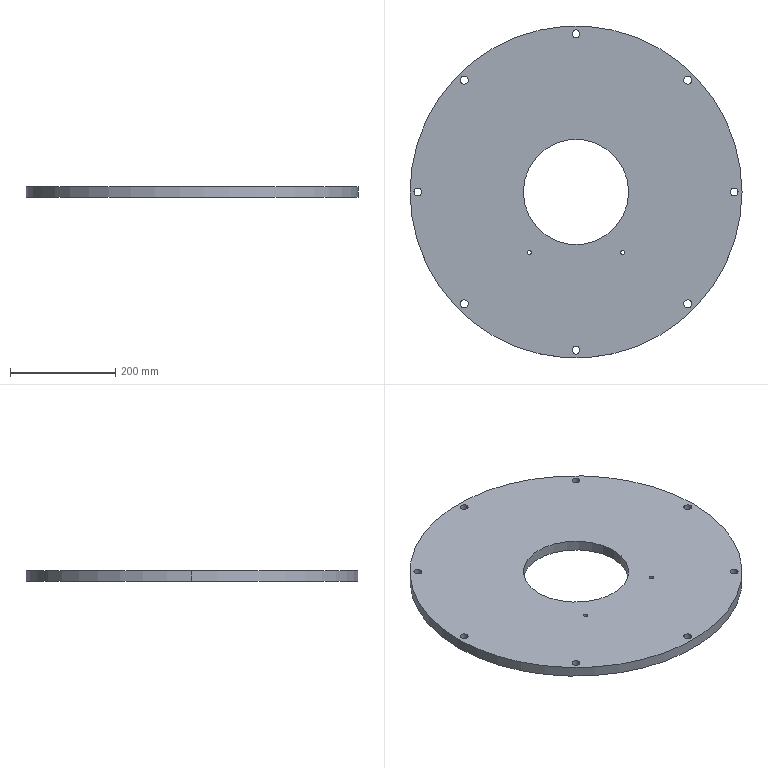Part | SolidWorks | features Cut 1, Extrusion 1 | 1 solid | 26 faces | box 630 x 630 x 20 mm | volume 5575887 mm3 | cylinder 24 | plane 2 | commonest cylinder face diameters 15 x16 8 x4 200 x2 630 x2
STEP:
#1=CARTESIAN_POINT('',(84.459,-114.891,20.));
#2=VERTEX_POINT('',#1);
#3=CARTESIAN_POINT('',(92.459,-114.891,20.));
#4=VERTEX_POINT('',#3);
#5=CARTESIAN_POINT('',(88.459,-114.891,20.));
#6=DIRECTION('',(0.,0.,1.));
#7=DIRECTION('',(1.,0.,0.));
#8=AXIS2_PLACEMENT_3D('',#5,#6,#7);
#9=CIRCLE('',#8,4.);
#10=EDGE_CURVE('',#2,#4,#9,.T.);
#11=ORIENTED_EDGE('',*,*,#10,.T.);
#12=CARTESIAN_POINT('',(92.459,-114.891,0.));
#13=VERTEX_POINT('',#12);
#14=CARTESIAN_POINT('',(92.459,-114.891,50.));
#15=DIRECTION('',(0.,0.,-1.));
#16=VECTOR('',#15,1000.);
#17=LINE('',#14,#16);
#18=EDGE_CURVE('',#4,#13,#17,.T.);
#19=ORIENTED_EDGE('',*,*,#18,.T.);
#20=CARTESIAN_POINT('',(84.459,-114.891,0.));
#21=VERTEX_POINT('',#20);
#22=CARTESIAN_POINT('',(88.459,-114.891,0.));
#23=DIRECTION('',(0.,0.,-1.));
#24=DIRECTION('',(-1.,0.,0.));
#25=AXIS2_PLACEMENT_3D('',#22,#23,#24);
#26=CIRCLE('',#25,4.);
#27=EDGE_CURVE('',#13,#21,#26,.T.);
#28=ORIENTED_EDGE('',*,*,#27,.T.);
#29=CARTESIAN_POINT('',(84.459,-114.891,50.));
#30=DIRECTION('',(0.,0.,-1.));
#31=VECTOR('',#30,1000.);
#32=LINE('',#29,#31);
#33=EDGE_CURVE('',#2,#21,#32,.T.);
#34=ORIENTED_EDGE('',*,*,#33,.F.);
#35=EDGE_LOOP('',(#11,#19,#28,#34));
#36=FACE_OUTER_BOUND('',#35,.T.);
#37=CARTESIAN_POINT('',(88.459,-114.891,50.));
#38=DIRECTION('',(0.,0.,-1.));
#39=DIRECTION('',(-1.,0.,0.));
#40=AXIS2_PLACEMENT_3D('',#37,#38,#39);
#41=CYLINDRICAL_SURFACE('',#40,4.);
#42=ADVANCED_FACE('',(#36),#41,.F.);
#43=CARTESIAN_POINT('',(-92.459,-114.891,20.));
#44=VERTEX_POINT('',#43);
#45=CARTESIAN_POINT('',(-84.459,-114.891,20.));
#46=VERTEX_POINT('',#45);
#47=CARTESIAN_POINT('',(-88.459,-114.891,20.));
#48=DIRECTION('',(0.,0.,1.));
#49=DIRECTION('',(1.,0.,0.));
#50=AXIS2_PLACEMENT_3D('',#47,#48,#49);
#51=CIRCLE('',#50,4.);
#52=EDGE_CURVE('',#44,#46,#51,.T.);
#53=ORIENTED_EDGE('',*,*,#52,.T.);
#54=CARTESIAN_POINT('',(-84.459,-114.891,0.));
#55=VERTEX_POINT('',#54);
#56=CARTESIAN_POINT('',(-84.459,-114.891,50.));
#57=DIRECTION('',(0.,0.,-1.));
#58=VECTOR('',#57,1000.);
#59=LINE('',#56,#58);
#60=EDGE_CURVE('',#46,#55,#59,.T.);
#61=ORIENTED_EDGE('',*,*,#60,.T.);
#62=CARTESIAN_POINT('',(-92.459,-114.891,0.));
#63=VERTEX_POINT('',#62);
#64=CARTESIAN_POINT('',(-88.459,-114.891,0.));
#65=DIRECTION('',(0.,0.,-1.));
#66=DIRECTION('',(-1.,0.,0.));
#67=AXIS2_PLACEMENT_3D('',#64,#65,#66);
#68=CIRCLE('',#67,4.);
#69=EDGE_CURVE('',#55,#63,#68,.T.);
#70=ORIENTED_EDGE('',*,*,#69,.T.);
#71=CARTESIAN_POINT('',(-92.459,-114.891,50.));
#72=DIRECTION('',(0.,0.,-1.));
#73=VECTOR('',#72,1000.);
#74=LINE('',#71,#73);
#75=EDGE_CURVE('',#44,#63,#74,.T.);
#76=ORIENTED_EDGE('',*,*,#75,.F.);
#77=EDGE_LOOP('',(#53,#61,#70,#76));
#78=FACE_OUTER_BOUND('',#77,.T.);
#79=CARTESIAN_POINT('',(-88.459,-114.891,50.));
#80=DIRECTION('',(0.,0.,-1.));
#81=DIRECTION('',(-1.,0.,0.));
#82=AXIS2_PLACEMENT_3D('',#79,#80,#81);
#83=CYLINDRICAL_SURFACE('',#82,4.);
#84=ADVANCED_FACE('',(#78),#83,.F.);
#85=CARTESIAN_POINT('',(-219.632,212.132,20.));
#86=VERTEX_POINT('',#85);
#87=CARTESIAN_POINT('',(-204.632,212.132,20.));
#88=VERTEX_POINT('',#87);
#89=CARTESIAN_POINT('',(-212.132,212.132,20.));
#90=DIRECTION('',(0.,0.,1.));
#91=DIRECTION('',(1.,0.,0.));
#92=AXIS2_PLACEMENT_3D('',#89,#90,#91);
#93=CIRCLE('',#92,7.5);
#94=EDGE_CURVE('',#86,#88,#93,.T.);
#95=ORIENTED_EDGE('',*,*,#94,.T.);
#96=CARTESIAN_POINT('',(-204.632,212.132,0.));
#97=VERTEX_POINT('',#96);
#98=CARTESIAN_POINT('',(-204.632,212.132,20.));
#99=DIRECTION('',(0.,0.,-1.));
#100=VECTOR('',#99,1000.);
#101=LINE('',#98,#100);
#102=EDGE_CURVE('',#88,#97,#101,.T.);
#103=ORIENTED_EDGE('',*,*,#102,.T.);
#104=CARTESIAN_POINT('',(-219.632,212.132,0.));
#105=VERTEX_POINT('',#104);
#106=CARTESIAN_POINT('',(-212.132,212.132,0.));
#107=DIRECTION('',(0.,0.,1.));
#108=DIRECTION('',(1.,0.,0.));
#109=AXIS2_PLACEMENT_3D('',#106,#107,#108);
#110=CIRCLE('',#109,7.5);
#111=EDGE_CURVE('',#105,#97,#110,.T.);
#112=ORIENTED_EDGE('',*,*,#111,.F.);
#113=CARTESIAN_POINT('',(-219.632,212.132,20.));
#114=DIRECTION('',(0.,0.,-1.));
#115=VECTOR('',#114,1000.);
#116=LINE('',#113,#115);
#117=EDGE_CURVE('',#86,#105,#116,.T.);
#118=ORIENTED_EDGE('',*,*,#117,.F.);
#119=EDGE_LOOP('',(#95,#103,#112,#118));
#120=FACE_OUTER_BOUND('',#119,.T.);
#121=CARTESIAN_POINT('',(-212.132,212.132,20.));
#122=DIRECTION('',(0.,0.,-1.));
#123=DIRECTION('',(-1.,0.,0.));
#124=AXIS2_PLACEMENT_3D('',#121,#122,#123);
#125=CYLINDRICAL_SURFACE('',#124,7.5);
#126=ADVANCED_FACE('',(#120),#125,.F.);
#127=CARTESIAN_POINT('',(-307.5,0.,20.));
#128=VERTEX_POINT('',#127);
#129=CARTESIAN_POINT('',(-292.5,0.,20.));
#130=VERTEX_POINT('',#129);
#131=CARTESIAN_POINT('',(-300.,0.,20.));
#132=DIRECTION('',(0.,0.,1.));
#133=DIRECTION('',(1.,0.,0.));
#134=AXIS2_PLACEMENT_3D('',#131,#132,#133);
#135=CIRCLE('',#134,7.5);
#136=EDGE_CURVE('',#128,#130,#135,.T.);
#137=ORIENTED_EDGE('',*,*,#136,.T.);
#138=CARTESIAN_POINT('',(-292.5,0.,0.));
#139=VERTEX_POINT('',#138);
#140=CARTESIAN_POINT('',(-292.5,0.,20.));
#141=DIRECTION('',(0.,0.,-1.));
#142=VECTOR('',#141,1000.);
#143=LINE('',#140,#142);
#144=EDGE_CURVE('',#130,#139,#143,.T.);
#145=ORIENTED_EDGE('',*,*,#144,.T.);
#146=CARTESIAN_POINT('',(-307.5,0.,0.));
#147=VERTEX_POINT('',#146);
#148=CARTESIAN_POINT('',(-300.,0.,0.));
#149=DIRECTION('',(0.,0.,1.));
#150=DIRECTION('',(1.,0.,0.));
#151=AXIS2_PLACEMENT_3D('',#148,#149,#150);
#152=CIRCLE('',#151,7.5);
#153=EDGE_CURVE('',#147,#139,#152,.T.);
#154=ORIENTED_EDGE('',*,*,#153,.F.);
#155=CARTESIAN_POINT('',(-307.5,0.,20.));
#156=DIRECTION('',(0.,0.,-1.));
#157=VECTOR('',#156,1000.);
#158=LINE('',#155,#157);
#159=EDGE_CURVE('',#128,#147,#158,.T.);
#160=ORIENTED_EDGE('',*,*,#159,.F.);
#161=EDGE_LOOP('',(#137,#145,#154,#160));
#162=FACE_OUTER_BOUND('',#161,.T.);
#163=CARTESIAN_POINT('',(-300.,0.,20.));
#164=DIRECTION('',(0.,0.,-1.));
#165=DIRECTION('',(-1.,0.,0.));
#166=AXIS2_PLACEMENT_3D('',#163,#164,#165);
#167=CYLINDRICAL_SURFACE('',#166,7.5);
#168=ADVANCED_FACE('',(#162),#167,.F.);
#169=CARTESIAN_POINT('',(-219.632,-212.132,20.));
#170=VERTEX_POINT('',#169);
#171=CARTESIAN_POINT('',(-204.632,-212.132,20.));
#172=VERTEX_POINT('',#171);
#173=CARTESIAN_POINT('',(-212.132,-212.132,20.));
#174=DIRECTION('',(0.,0.,1.));
#175=DIRECTION('',(1.,0.,0.));
#176=AXIS2_PLACEMENT_3D('',#173,#174,#175);
#177=CIRCLE('',#176,7.5);
#178=EDGE_CURVE('',#170,#172,#177,.T.);
#179=ORIENTED_EDGE('',*,*,#178,.T.);
#180=CARTESIAN_POINT('',(-204.632,-212.132,0.));
#181=VERTEX_POINT('',#180);
#182=CARTESIAN_POINT('',(-204.632,-212.132,20.));
#183=DIRECTION('',(0.,0.,-1.));
#184=VECTOR('',#183,1000.);
#185=LINE('',#182,#184);
#186=EDGE_CURVE('',#172,#181,#185,.T.);
#187=ORIENTED_EDGE('',*,*,#186,.T.);
#188=CARTESIAN_POINT('',(-219.632,-212.132,0.));
#189=VERTEX_POINT('',#188);
#190=CARTESIAN_POINT('',(-212.132,-212.132,0.));
#191=DIRECTION('',(0.,0.,1.));
#192=DIRECTION('',(1.,0.,0.));
#193=AXIS2_PLACEMENT_3D('',#190,#191,#192);
#194=CIRCLE('',#193,7.5);
#195=EDGE_CURVE('',#189,#181,#194,.T.);
#196=ORIENTED_EDGE('',*,*,#195,.F.);
#197=CARTESIAN_POINT('',(-219.632,-212.132,20.));
#198=DIRECTION('',(0.,0.,-1.));
#199=VECTOR('',#198,1000.);
#200=LINE('',#197,#199);
#201=EDGE_CURVE('',#170,#189,#200,.T.);
#202=ORIENTED_EDGE('',*,*,#201,.F.);
#203=EDGE_LOOP('',(#179,#187,#196,#202));
#204=FACE_OUTER_BOUND('',#203,.T.);
#205=CARTESIAN_POINT('',(-212.132,-212.132,20.));
#206=DIRECTION('',(0.,0.,-1.));
#207=DIRECTION('',(-1.,0.,0.));
#208=AXIS2_PLACEMENT_3D('',#205,#206,#207);
#209=CYLINDRICAL_SURFACE('',#208,7.5);
#210=ADVANCED_FACE('',(#204),#209,.F.);
#211=CARTESIAN_POINT('',(-7.5,-300.,20.));
#212=VERTEX_POINT('',#211);
#213=CARTESIAN_POINT('',(7.5,-300.,20.));
#214=VERTEX_POINT('',#213);
#215=CARTESIAN_POINT('',(0.,-300.,20.));
#216=DIRECTION('',(0.,0.,1.));
#217=DIRECTION('',(1.,0.,0.));
#218=AXIS2_PLACEMENT_3D('',#215,#216,#217);
#219=CIRCLE('',#218,7.5);
#220=EDGE_CURVE('',#212,#214,#219,.T.);
#221=ORIENTED_EDGE('',*,*,#220,.T.);
#222=CARTESIAN_POINT('',(7.5,-300.,0.));
#223=VERTEX_POINT('',#222);
#224=CARTESIAN_POINT('',(7.5,-300.,20.));
#225=DIRECTION('',(0.,0.,-1.));
#226=VECTOR('',#225,1000.);
#227=LINE('',#224,#226);
#228=EDGE_CURVE('',#214,#223,#227,.T.);
#229=ORIENTED_EDGE('',*,*,#228,.T.);
#230=CARTESIAN_POINT('',(-7.5,-300.,0.));
#231=VERTEX_POINT('',#230);
#232=CARTESIAN_POINT('',(0.,-300.,0.));
#233=DIRECTION('',(0.,0.,1.));
#234=DIRECTION('',(1.,0.,0.));
#235=AXIS2_PLACEMENT_3D('',#232,#233,#234);
#236=CIRCLE('',#235,7.5);
#237=EDGE_CURVE('',#231,#223,#236,.T.);
#238=ORIENTED_EDGE('',*,*,#237,.F.);
#239=CARTESIAN_POINT('',(-7.5,-300.,20.));
#240=DIRECTION('',(0.,0.,-1.));
#241=VECTOR('',#240,1000.);
#242=LINE('',#239,#241);
#243=EDGE_CURVE('',#212,#231,#242,.T.);
#244=ORIENTED_EDGE('',*,*,#243,.F.);
#245=EDGE_LOOP('',(#221,#229,#238,#244));
#246=FACE_OUTER_BOUND('',#245,.T.);
#247=CARTESIAN_POINT('',(0.,-300.,20.));
#248=DIRECTION('',(0.,0.,-1.));
#249=DIRECTION('',(-1.,0.,0.));
#250=AXIS2_PLACEMENT_3D('',#247,#248,#249);
#251=CYLINDRICAL_SURFACE('',#250,7.5);
#252=ADVANCED_FACE('',(#246),#251,.F.);
#253=CARTESIAN_POINT('',(204.632,-212.132,20.));
#254=VERTEX_POINT('',#253);
#255=CARTESIAN_POINT('',(219.632,-212.132,20.));
#256=VERTEX_POINT('',#255);
#257=CARTESIAN_POINT('',(212.132,-212.132,20.));
#258=DIRECTION('',(0.,0.,1.));
#259=DIRECTION('',(1.,0.,0.));
#260=AXIS2_PLACEMENT_3D('',#257,#258,#259);
#261=CIRCLE('',#260,7.5);
#262=EDGE_CURVE('',#254,#256,#261,.T.);
#263=ORIENTED_EDGE('',*,*,#262,.T.);
#264=CARTESIAN_POINT('',(219.632,-212.132,0.));
#265=VERTEX_POINT('',#264);
#266=CARTESIAN_POINT('',(219.632,-212.132,20.));
#267=DIRECTION('',(0.,0.,-1.));
#268=VECTOR('',#267,1000.);
#269=LINE('',#266,#268);
#270=EDGE_CURVE('',#256,#265,#269,.T.);
#271=ORIENTED_EDGE('',*,*,#270,.T.);
#272=CARTESIAN_POINT('',(204.632,-212.132,0.));
#273=VERTEX_POINT('',#272);
#274=CARTESIAN_POINT('',(212.132,-212.132,0.));
#275=DIRECTION('',(0.,0.,1.));
#276=DIRECTION('',(1.,0.,0.));
#277=AXIS2_PLACEMENT_3D('',#274,#275,#276);
#278=CIRCLE('',#277,7.5);
#279=EDGE_CURVE('',#273,#265,#278,.T.);
#280=ORIENTED_EDGE('',*,*,#279,.F.);
#281=CARTESIAN_POINT('',(204.632,-212.132,20.));
#282=DIRECTION('',(0.,0.,-1.));
#283=VECTOR('',#282,1000.);
#284=LINE('',#281,#283);
#285=EDGE_CURVE('',#254,#273,#284,.T.);
#286=ORIENTED_EDGE('',*,*,#285,.F.);
#287=EDGE_LOOP('',(#263,#271,#280,#286));
#288=FACE_OUTER_BOUND('',#287,.T.);
#289=CARTESIAN_POINT('',(212.132,-212.132,20.));
#290=DIRECTION('',(0.,0.,-1.));
#291=DIRECTION('',(-1.,0.,0.));
#292=AXIS2_PLACEMENT_3D('',#289,#290,#291);
#293=CYLINDRICAL_SURFACE('',#292,7.5);
#294=ADVANCED_FACE('',(#288),#293,.F.);
#295=CARTESIAN_POINT('',(292.5,0.,20.));
#296=VERTEX_POINT('',#295);
#297=CARTESIAN_POINT('',(307.5,0.,20.));
#298=VERTEX_POINT('',#297);
#299=CARTESIAN_POINT('',(300.,0.,20.));
#300=DIRECTION('',(0.,0.,1.));
#301=DIRECTION('',(1.,0.,0.));
#302=AXIS2_PLACEMENT_3D('',#299,#300,#301);
#303=CIRCLE('',#302,7.5);
#304=EDGE_CURVE('',#296,#298,#303,.T.);
#305=ORIENTED_EDGE('',*,*,#304,.T.);
#306=CARTESIAN_POINT('',(307.5,0.,0.));
#307=VERTEX_POINT('',#306);
#308=CARTESIAN_POINT('',(307.5,0.,20.));
#309=DIRECTION('',(0.,0.,-1.));
#310=VECTOR('',#309,1000.);
#311=LINE('',#308,#310);
#312=EDGE_CURVE('',#298,#307,#311,.T.);
#313=ORIENTED_EDGE('',*,*,#312,.T.);
#314=CARTESIAN_POINT('',(292.5,0.,0.));
#315=VERTEX_POINT('',#314);
#316=CARTESIAN_POINT('',(300.,0.,0.));
#317=DIRECTION('',(0.,0.,1.));
#318=DIRECTION('',(1.,0.,0.));
#319=AXIS2_PLACEMENT_3D('',#316,#317,#318);
#320=CIRCLE('',#319,7.5);
#321=EDGE_CURVE('',#315,#307,#320,.T.);
#322=ORIENTED_EDGE('',*,*,#321,.F.);
#323=CARTESIAN_POINT('',(292.5,0.,20.));
#324=DIRECTION('',(0.,0.,-1.));
#325=VECTOR('',#324,1000.);
#326=LINE('',#323,#325);
#327=EDGE_CURVE('',#296,#315,#326,.T.);
#328=ORIENTED_EDGE('',*,*,#327,.F.);
#329=EDGE_LOOP('',(#305,#313,#322,#328));
#330=FACE_OUTER_BOUND('',#329,.T.);
#331=CARTESIAN_POINT('',(300.,0.,20.));
#332=DIRECTION('',(0.,0.,-1.));
#333=DIRECTION('',(-1.,0.,0.));
#334=AXIS2_PLACEMENT_3D('',#331,#332,#333);
#335=CYLINDRICAL_SURFACE('',#334,7.5);
#336=ADVANCED_FACE('',(#330),#335,.F.);
#337=CARTESIAN_POINT('',(204.632,212.132,20.));
#338=VERTEX_POINT('',#337);
#339=CARTESIAN_POINT('',(219.632,212.132,20.));
#340=VERTEX_POINT('',#339);
#341=CARTESIAN_POINT('',(212.132,212.132,20.));
#342=DIRECTION('',(0.,0.,1.));
#343=DIRECTION('',(1.,0.,0.));
#344=AXIS2_PLACEMENT_3D('',#341,#342,#343);
#345=CIRCLE('',#344,7.5);
#346=EDGE_CURVE('',#338,#340,#345,.T.);
#347=ORIENTED_EDGE('',*,*,#346,.T.);
#348=CARTESIAN_POINT('',(219.632,212.132,0.));
#349=VERTEX_POINT('',#348);
#350=CARTESIAN_POINT('',(219.632,212.132,20.));
#351=DIRECTION('',(0.,0.,-1.));
#352=VECTOR('',#351,1000.);
#353=LINE('',#350,#352);
#354=EDGE_CURVE('',#340,#349,#353,.T.);
#355=ORIENTED_EDGE('',*,*,#354,.T.);
#356=CARTESIAN_POINT('',(204.632,212.132,0.));
#357=VERTEX_POINT('',#356);
#358=CARTESIAN_POINT('',(212.132,212.132,0.));
#359=DIRECTION('',(0.,0.,1.));
#360=DIRECTION('',(1.,0.,0.));
#361=AXIS2_PLACEMENT_3D('',#358,#359,#360);
#362=CIRCLE('',#361,7.5);
#363=EDGE_CURVE('',#357,#349,#362,.T.);
#364=ORIENTED_EDGE('',*,*,#363,.F.);
#365=CARTESIAN_POINT('',(204.632,212.132,20.));
#366=DIRECTION('',(0.,0.,-1.));
#367=VECTOR('',#366,1000.);
#368=LINE('',#365,#367);
#369=EDGE_CURVE('',#338,#357,#368,.T.);
#370=ORIENTED_EDGE('',*,*,#369,.F.);
#371=EDGE_LOOP('',(#347,#355,#364,#370));
#372=FACE_OUTER_BOUND('',#371,.T.);
#373=CARTESIAN_POINT('',(212.132,212.132,20.));
#374=DIRECTION('',(0.,0.,-1.));
#375=DIRECTION('',(-1.,0.,0.));
#376=AXIS2_PLACEMENT_3D('',#373,#374,#375);
#377=CYLINDRICAL_SURFACE('',#376,7.5);
#378=ADVANCED_FACE('',(#372),#377,.F.);
#379=CARTESIAN_POINT('',(-7.5,300.,20.));
#380=VERTEX_POINT('',#379);
#381=CARTESIAN_POINT('',(7.5,300.,20.));
#382=VERTEX_POINT('',#381);
#383=CARTESIAN_POINT('',(0.,300.,20.));
#384=DIRECTION('',(0.,0.,1.));
#385=DIRECTION('',(1.,0.,0.));
#386=AXIS2_PLACEMENT_3D('',#383,#384,#385);
#387=CIRCLE('',#386,7.5);
#388=EDGE_CURVE('',#380,#382,#387,.T.);
#389=ORIENTED_EDGE('',*,*,#388,.T.);
#390=CARTESIAN_POINT('',(7.5,300.,0.));
#391=VERTEX_POINT('',#390);
#392=CARTESIAN_POINT('',(7.5,300.,20.));
#393=DIRECTION('',(0.,0.,-1.));
#394=VECTOR('',#393,1000.);
#395=LINE('',#392,#394);
#396=EDGE_CURVE('',#382,#391,#395,.T.);
#397=ORIENTED_EDGE('',*,*,#396,.T.);
#398=CARTESIAN_POINT('',(-7.5,300.,0.));
#399=VERTEX_POINT('',#398);
#400=CARTESIAN_POINT('',(0.,300.,0.));
#401=DIRECTION('',(0.,0.,1.));
#402=DIRECTION('',(1.,0.,0.));
#403=AXIS2_PLACEMENT_3D('',#400,#401,#402);
#404=CIRCLE('',#403,7.5);
#405=EDGE_CURVE('',#399,#391,#404,.T.);
#406=ORIENTED_EDGE('',*,*,#405,.F.);
#407=CARTESIAN_POINT('',(-7.5,300.,20.));
#408=DIRECTION('',(0.,0.,-1.));
#409=VECTOR('',#408,1000.);
#410=LINE('',#407,#409);
#411=EDGE_CURVE('',#380,#399,#410,.T.);
#412=ORIENTED_EDGE('',*,*,#411,.F.);
#413=EDGE_LOOP('',(#389,#397,#406,#412));
#414=FACE_OUTER_BOUND('',#413,.T.);
#415=CARTESIAN_POINT('',(0.,300.,20.));
#416=DIRECTION('',(0.,0.,-1.));
#417=DIRECTION('',(-1.,0.,0.));
#418=AXIS2_PLACEMENT_3D('',#415,#416,#417);
#419=CYLINDRICAL_SURFACE('',#418,7.5);
#420=ADVANCED_FACE('',(#414),#419,.F.);
#421=CARTESIAN_POINT('',(-100.,0.,20.));
#422=VERTEX_POINT('',#421);
#423=CARTESIAN_POINT('',(100.,0.,20.));
#424=VERTEX_POINT('',#423);
#425=CARTESIAN_POINT('',(0.,0.,20.));
#426=DIRECTION('',(0.,0.,1.));
#427=DIRECTION('',(1.,0.,0.));
#428=AXIS2_PLACEMENT_3D('',#425,#426,#427);
#429=CIRCLE('',#428,100.);
#430=EDGE_CURVE('',#422,#424,#429,.T.);
#431=ORIENTED_EDGE('',*,*,#430,.T.);
#432=CARTESIAN_POINT('',(100.,0.,0.));
#433=VERTEX_POINT('',#432);
#434=CARTESIAN_POINT('',(100.,0.,20.));
#435=DIRECTION('',(0.,0.,-1.));
#436=VECTOR('',#435,1000.);
#437=LINE('',#434,#436);
#438=EDGE_CURVE('',#424,#433,#437,.T.);
#439=ORIENTED_EDGE('',*,*,#438,.T.);
#440=CARTESIAN_POINT('',(-100.,0.,0.));
#441=VERTEX_POINT('',#440);
#442=CARTESIAN_POINT('',(0.,0.,0.));
#443=DIRECTION('',(0.,0.,1.));
#444=DIRECTION('',(1.,0.,0.));
#445=AXIS2_PLACEMENT_3D('',#442,#443,#444);
#446=CIRCLE('',#445,100.);
#447=EDGE_CURVE('',#441,#433,#446,.T.);
#448=ORIENTED_EDGE('',*,*,#447,.F.);
#449=CARTESIAN_POINT('',(-100.,0.,20.));
#450=DIRECTION('',(0.,0.,-1.));
#451=VECTOR('',#450,1000.);
#452=LINE('',#449,#451);
#453=EDGE_CURVE('',#422,#441,#452,.T.);
#454=ORIENTED_EDGE('',*,*,#453,.F.);
#455=EDGE_LOOP('',(#431,#439,#448,#454));
#456=FACE_OUTER_BOUND('',#455,.T.);
#457=CARTESIAN_POINT('',(0.,0.,20.));
#458=DIRECTION('',(0.,0.,-1.));
#459=DIRECTION('',(-1.,0.,0.));
#460=AXIS2_PLACEMENT_3D('',#457,#458,#459);
#461=CYLINDRICAL_SURFACE('',#460,100.);
#462=ADVANCED_FACE('',(#456),#461,.F.);
#463=CARTESIAN_POINT('',(315.,0.,20.));
#464=VERTEX_POINT('',#463);
#465=CARTESIAN_POINT('',(-315.,0.,20.));
#466=VERTEX_POINT('',#465);
#467=CARTESIAN_POINT('',(0.,0.,20.));
#468=DIRECTION('',(0.,0.,1.));
#469=DIRECTION('',(1.,0.,0.));
#470=AXIS2_PLACEMENT_3D('',#467,#468,#469);
#471=CIRCLE('',#470,315.);
#472=EDGE_CURVE('',#464,#466,#471,.T.);
#473=ORIENTED_EDGE('',*,*,#472,.F.);
#474=CARTESIAN_POINT('',(315.,0.,0.));
#475=VERTEX_POINT('',#474);
#476=CARTESIAN_POINT('',(315.,0.,20.));
#477=DIRECTION('',(0.,0.,-1.));
#478=VECTOR('',#477,1000.);
#479=LINE('',#476,#478);
#480=EDGE_CURVE('',#464,#475,#479,.T.);
#481=ORIENTED_EDGE('',*,*,#480,.T.);
#482=CARTESIAN_POINT('',(-315.,0.,0.));
#483=VERTEX_POINT('',#482);
#484=CARTESIAN_POINT('',(0.,0.,0.));
#485=DIRECTION('',(0.,0.,1.));
#486=DIRECTION('',(1.,0.,0.));
#487=AXIS2_PLACEMENT_3D('',#484,#485,#486);
#488=CIRCLE('',#487,315.);
#489=EDGE_CURVE('',#475,#483,#488,.T.);
#490=ORIENTED_EDGE('',*,*,#489,.T.);
#491=CARTESIAN_POINT('',(-315.,0.,20.));
#492=DIRECTION('',(0.,0.,-1.));
#493=VECTOR('',#492,1000.);
#494=LINE('',#491,#493);
#495=EDGE_CURVE('',#466,#483,#494,.T.);
#496=ORIENTED_EDGE('',*,*,#495,.F.);
#497=EDGE_LOOP('',(#473,#481,#490,#496));
#498=FACE_OUTER_BOUND('',#497,.T.);
#499=CARTESIAN_POINT('',(0.,0.,20.));
#500=DIRECTION('',(0.,0.,-1.));
#501=DIRECTION('',(-1.,0.,0.));
#502=AXIS2_PLACEMENT_3D('',#499,#500,#501);
#503=CYLINDRICAL_SURFACE('',#502,315.);
#504=ADVANCED_FACE('',(#498),#503,.T.);
#505=ORIENTED_EDGE('',*,*,#10,.F.);
#506=CARTESIAN_POINT('',(88.459,-114.891,20.));
#507=DIRECTION('',(0.,0.,1.));
#508=DIRECTION('',(1.,0.,0.));
#509=AXIS2_PLACEMENT_3D('',#506,#507,#508);
#510=CIRCLE('',#509,4.);
#511=EDGE_CURVE('',#4,#2,#510,.T.);
#512=ORIENTED_EDGE('',*,*,#511,.F.);
#513=EDGE_LOOP('',(#505,#512));
#514=FACE_BOUND('',#513,.T.);
#515=ORIENTED_EDGE('',*,*,#52,.F.);
#516=CARTESIAN_POINT('',(-88.459,-114.891,20.));
#517=DIRECTION('',(0.,0.,1.));
#518=DIRECTION('',(1.,0.,0.));
#519=AXIS2_PLACEMENT_3D('',#516,#517,#518);
#520=CIRCLE('',#519,4.);
#521=EDGE_CURVE('',#46,#44,#520,.T.);
#522=ORIENTED_EDGE('',*,*,#521,.F.);
#523=EDGE_LOOP('',(#515,#522));
#524=FACE_BOUND('',#523,.T.);
#525=ORIENTED_EDGE('',*,*,#136,.F.);
#526=CARTESIAN_POINT('',(-300.,0.,20.));
#527=DIRECTION('',(0.,0.,1.));
#528=DIRECTION('',(1.,0.,0.));
#529=AXIS2_PLACEMENT_3D('',#526,#527,#528);
#530=CIRCLE('',#529,7.5);
#531=EDGE_CURVE('',#130,#128,#530,.T.);
#532=ORIENTED_EDGE('',*,*,#531,.F.);
#533=EDGE_LOOP('',(#525,#532));
#534=FACE_BOUND('',#533,.T.);
#535=ORIENTED_EDGE('',*,*,#220,.F.);
#536=CARTESIAN_POINT('',(0.,-300.,20.));
#537=DIRECTION('',(0.,0.,1.));
#538=DIRECTION('',(1.,0.,0.));
#539=AXIS2_PLACEMENT_3D('',#536,#537,#538);
#540=CIRCLE('',#539,7.5);
#541=EDGE_CURVE('',#214,#212,#540,.T.);
#542=ORIENTED_EDGE('',*,*,#541,.F.);
#543=EDGE_LOOP('',(#535,#542));
#544=FACE_BOUND('',#543,.T.);
#545=ORIENTED_EDGE('',*,*,#304,.F.);
#546=CARTESIAN_POINT('',(300.,0.,20.));
#547=DIRECTION('',(0.,0.,1.));
#548=DIRECTION('',(1.,0.,0.));
#549=AXIS2_PLACEMENT_3D('',#546,#547,#548);
#550=CIRCLE('',#549,7.5);
#551=EDGE_CURVE('',#298,#296,#550,.T.);
#552=ORIENTED_EDGE('',*,*,#551,.F.);
#553=EDGE_LOOP('',(#545,#552));
#554=FACE_BOUND('',#553,.T.);
#555=ORIENTED_EDGE('',*,*,#388,.F.);
#556=CARTESIAN_POINT('',(0.,300.,20.));
#557=DIRECTION('',(0.,0.,1.));
#558=DIRECTION('',(1.,0.,0.));
#559=AXIS2_PLACEMENT_3D('',#556,#557,#558);
#560=CIRCLE('',#559,7.5);
#561=EDGE_CURVE('',#382,#380,#560,.T.);
#562=ORIENTED_EDGE('',*,*,#561,.F.);
#563=EDGE_LOOP('',(#555,#562));
#564=FACE_BOUND('',#563,.T.);
#565=CARTESIAN_POINT('',(0.,0.,20.));
#566=DIRECTION('',(0.,0.,1.));
#567=DIRECTION('',(1.,0.,0.));
#568=AXIS2_PLACEMENT_3D('',#565,#566,#567);
#569=CIRCLE('',#568,315.);
#570=EDGE_CURVE('',#466,#464,#569,.T.);
#571=ORIENTED_EDGE('',*,*,#570,.T.);
#572=ORIENTED_EDGE('',*,*,#472,.T.);
#573=EDGE_LOOP('',(#571,#572));
#574=FACE_OUTER_BOUND('',#573,.T.);
#575=ORIENTED_EDGE('',*,*,#430,.F.);
#576=CARTESIAN_POINT('',(0.,0.,20.));
#577=DIRECTION('',(0.,0.,1.));
#578=DIRECTION('',(1.,0.,0.));
#579=AXIS2_PLACEMENT_3D('',#576,#577,#578);
#580=CIRCLE('',#579,100.);
#581=EDGE_CURVE('',#424,#422,#580,.T.);
#582=ORIENTED_EDGE('',*,*,#581,.F.);
#583=EDGE_LOOP('',(#575,#582));
#584=FACE_BOUND('',#583,.T.);
#585=ORIENTED_EDGE('',*,*,#346,.F.);
#586=CARTESIAN_POINT('',(212.132,212.132,20.));
#587=DIRECTION('',(0.,0.,1.));
#588=DIRECTION('',(1.,0.,0.));
#589=AXIS2_PLACEMENT_3D('',#586,#587,#588);
#590=CIRCLE('',#589,7.5);
#591=EDGE_CURVE('',#340,#338,#590,.T.);
#592=ORIENTED_EDGE('',*,*,#591,.F.);
#593=EDGE_LOOP('',(#585,#592));
#594=FACE_BOUND('',#593,.T.);
#595=ORIENTED_EDGE('',*,*,#262,.F.);
#596=CARTESIAN_POINT('',(212.132,-212.132,20.));
#597=DIRECTION('',(0.,0.,1.));
#598=DIRECTION('',(1.,0.,0.));
#599=AXIS2_PLACEMENT_3D('',#596,#597,#598);
#600=CIRCLE('',#599,7.5);
#601=EDGE_CURVE('',#256,#254,#600,.T.);
#602=ORIENTED_EDGE('',*,*,#601,.F.);
#603=EDGE_LOOP('',(#595,#602));
#604=FACE_BOUND('',#603,.T.);
#605=ORIENTED_EDGE('',*,*,#178,.F.);
#606=CARTESIAN_POINT('',(-212.132,-212.132,20.));
#607=DIRECTION('',(0.,0.,1.));
#608=DIRECTION('',(1.,0.,0.));
#609=AXIS2_PLACEMENT_3D('',#606,#607,#608);
#610=CIRCLE('',#609,7.5);
#611=EDGE_CURVE('',#172,#170,#610,.T.);
#612=ORIENTED_EDGE('',*,*,#611,.F.);
#613=EDGE_LOOP('',(#605,#612));
#614=FACE_BOUND('',#613,.T.);
#615=ORIENTED_EDGE('',*,*,#94,.F.);
#616=CARTESIAN_POINT('',(-212.132,212.132,20.));
#617=DIRECTION('',(0.,0.,1.));
#618=DIRECTION('',(1.,0.,0.));
#619=AXIS2_PLACEMENT_3D('',#616,#617,#618);
#620=CIRCLE('',#619,7.5);
#621=EDGE_CURVE('',#88,#86,#620,.T.);
#622=ORIENTED_EDGE('',*,*,#621,.F.);
#623=EDGE_LOOP('',(#615,#622));
#624=FACE_BOUND('',#623,.T.);
#625=CARTESIAN_POINT('',(0.,0.,20.));
#626=DIRECTION('',(0.,0.,1.));
#627=DIRECTION('',(1.,0.,0.));
#628=AXIS2_PLACEMENT_3D('',#625,#626,#627);
#629=PLANE('',#628);
#630=ADVANCED_FACE('',(#514,#524,#534,#544,#554,#564,#574,#584,#594,#604,#614,#624),#629,.T.);
#631=CARTESIAN_POINT('',(88.459,-114.891,0.));
#632=DIRECTION('',(0.,0.,-1.));
#633=DIRECTION('',(-1.,0.,0.));
#634=AXIS2_PLACEMENT_3D('',#631,#632,#633);
#635=CIRCLE('',#634,4.);
#636=EDGE_CURVE('',#21,#13,#635,.T.);
#637=ORIENTED_EDGE('',*,*,#636,.F.);
#638=ORIENTED_EDGE('',*,*,#27,.F.);
#639=EDGE_LOOP('',(#637,#638));
#640=FACE_BOUND('',#639,.T.);
#641=CARTESIAN_POINT('',(-88.459,-114.891,0.));
#642=DIRECTION('',(0.,0.,-1.));
#643=DIRECTION('',(-1.,0.,0.));
#644=AXIS2_PLACEMENT_3D('',#641,#642,#643);
#645=CIRCLE('',#644,4.);
#646=EDGE_CURVE('',#63,#55,#645,.T.);
#647=ORIENTED_EDGE('',*,*,#646,.F.);
#648=ORIENTED_EDGE('',*,*,#69,.F.);
#649=EDGE_LOOP('',(#647,#648));
#650=FACE_BOUND('',#649,.T.);
#651=CARTESIAN_POINT('',(0.,0.,0.));
#652=DIRECTION('',(0.,0.,1.));
#653=DIRECTION('',(1.,0.,0.));
#654=AXIS2_PLACEMENT_3D('',#651,#652,#653);
#655=CIRCLE('',#654,315.);
#656=EDGE_CURVE('',#483,#475,#655,.T.);
#657=ORIENTED_EDGE('',*,*,#656,.F.);
#658=ORIENTED_EDGE('',*,*,#489,.F.);
#659=EDGE_LOOP('',(#657,#658));
#660=FACE_OUTER_BOUND('',#659,.T.);
#661=ORIENTED_EDGE('',*,*,#447,.T.);
#662=CARTESIAN_POINT('',(0.,0.,0.));
#663=DIRECTION('',(0.,0.,1.));
#664=DIRECTION('',(1.,0.,0.));
#665=AXIS2_PLACEMENT_3D('',#662,#663,#664);
#666=CIRCLE('',#665,100.);
#667=EDGE_CURVE('',#433,#441,#666,.T.);
#668=ORIENTED_EDGE('',*,*,#667,.T.);
#669=EDGE_LOOP('',(#661,#668));
#670=FACE_BOUND('',#669,.T.);
#671=ORIENTED_EDGE('',*,*,#405,.T.);
#672=CARTESIAN_POINT('',(0.,300.,0.));
#673=DIRECTION('',(0.,0.,1.));
#674=DIRECTION('',(1.,0.,0.));
#675=AXIS2_PLACEMENT_3D('',#672,#673,#674);
#676=CIRCLE('',#675,7.5);
#677=EDGE_CURVE('',#391,#399,#676,.T.);
#678=ORIENTED_EDGE('',*,*,#677,.T.);
#679=EDGE_LOOP('',(#671,#678));
#680=FACE_BOUND('',#679,.T.);
#681=ORIENTED_EDGE('',*,*,#363,.T.);
#682=CARTESIAN_POINT('',(212.132,212.132,0.));
#683=DIRECTION('',(0.,0.,1.));
#684=DIRECTION('',(1.,0.,0.));
#685=AXIS2_PLACEMENT_3D('',#682,#683,#684);
#686=CIRCLE('',#685,7.5);
#687=EDGE_CURVE('',#349,#357,#686,.T.);
#688=ORIENTED_EDGE('',*,*,#687,.T.);
#689=EDGE_LOOP('',(#681,#688));
#690=FACE_BOUND('',#689,.T.);
#691=ORIENTED_EDGE('',*,*,#321,.T.);
#692=CARTESIAN_POINT('',(300.,0.,0.));
#693=DIRECTION('',(0.,0.,1.));
#694=DIRECTION('',(1.,0.,0.));
#695=AXIS2_PLACEMENT_3D('',#692,#693,#694);
#696=CIRCLE('',#695,7.5);
#697=EDGE_CURVE('',#307,#315,#696,.T.);
#698=ORIENTED_EDGE('',*,*,#697,.T.);
#699=EDGE_LOOP('',(#691,#698));
#700=FACE_BOUND('',#699,.T.);
#701=ORIENTED_EDGE('',*,*,#279,.T.);
#702=CARTESIAN_POINT('',(212.132,-212.132,0.));
#703=DIRECTION('',(0.,0.,1.));
#704=DIRECTION('',(1.,0.,0.));
#705=AXIS2_PLACEMENT_3D('',#702,#703,#704);
#706=CIRCLE('',#705,7.5);
#707=EDGE_CURVE('',#265,#273,#706,.T.);
#708=ORIENTED_EDGE('',*,*,#707,.T.);
#709=EDGE_LOOP('',(#701,#708));
#710=FACE_BOUND('',#709,.T.);
#711=ORIENTED_EDGE('',*,*,#237,.T.);
#712=CARTESIAN_POINT('',(0.,-300.,0.));
#713=DIRECTION('',(0.,0.,1.));
#714=DIRECTION('',(1.,0.,0.));
#715=AXIS2_PLACEMENT_3D('',#712,#713,#714);
#716=CIRCLE('',#715,7.5);
#717=EDGE_CURVE('',#223,#231,#716,.T.);
#718=ORIENTED_EDGE('',*,*,#717,.T.);
#719=EDGE_LOOP('',(#711,#718));
#720=FACE_BOUND('',#719,.T.);
#721=ORIENTED_EDGE('',*,*,#195,.T.);
#722=CARTESIAN_POINT('',(-212.132,-212.132,0.));
#723=DIRECTION('',(0.,0.,1.));
#724=DIRECTION('',(1.,0.,0.));
#725=AXIS2_PLACEMENT_3D('',#722,#723,#724);
#726=CIRCLE('',#725,7.5);
#727=EDGE_CURVE('',#181,#189,#726,.T.);
#728=ORIENTED_EDGE('',*,*,#727,.T.);
#729=EDGE_LOOP('',(#721,#728));
#730=FACE_BOUND('',#729,.T.);
#731=ORIENTED_EDGE('',*,*,#153,.T.);
#732=CARTESIAN_POINT('',(-300.,0.,0.));
#733=DIRECTION('',(0.,0.,1.));
#734=DIRECTION('',(1.,0.,0.));
#735=AXIS2_PLACEMENT_3D('',#732,#733,#734);
#736=CIRCLE('',#735,7.5);
#737=EDGE_CURVE('',#139,#147,#736,.T.);
#738=ORIENTED_EDGE('',*,*,#737,.T.);
#739=EDGE_LOOP('',(#731,#738));
#740=FACE_BOUND('',#739,.T.);
#741=ORIENTED_EDGE('',*,*,#111,.T.);
#742=CARTESIAN_POINT('',(-212.132,212.132,0.));
#743=DIRECTION('',(0.,0.,1.));
#744=DIRECTION('',(1.,0.,0.));
#745=AXIS2_PLACEMENT_3D('',#742,#743,#744);
#746=CIRCLE('',#745,7.5);
#747=EDGE_CURVE('',#97,#105,#746,.T.);
#748=ORIENTED_EDGE('',*,*,#747,.T.);
#749=EDGE_LOOP('',(#741,#748));
#750=FACE_BOUND('',#749,.T.);
#751=CARTESIAN_POINT('',(0.,0.,0.));
#752=DIRECTION('',(0.,0.,1.));
#753=DIRECTION('',(1.,0.,0.));
#754=AXIS2_PLACEMENT_3D('',#751,#752,#753);
#755=PLANE('',#754);
#756=ADVANCED_FACE('',(#640,#650,#660,#670,#680,#690,#700,#710,#720,#730,#740,#750),#755,.F.);
#757=ORIENTED_EDGE('',*,*,#480,.F.);
#758=ORIENTED_EDGE('',*,*,#570,.F.);
#759=ORIENTED_EDGE('',*,*,#495,.T.);
#760=ORIENTED_EDGE('',*,*,#656,.T.);
#761=EDGE_LOOP('',(#757,#758,#759,#760));
#762=FACE_OUTER_BOUND('',#761,.T.);
#763=CARTESIAN_POINT('',(0.,0.,20.));
#764=DIRECTION('',(0.,0.,-1.));
#765=DIRECTION('',(-1.,0.,0.));
#766=AXIS2_PLACEMENT_3D('',#763,#764,#765);
#767=CYLINDRICAL_SURFACE('',#766,315.);
#768=ADVANCED_FACE('',(#762),#767,.T.);
#769=ORIENTED_EDGE('',*,*,#438,.F.);
#770=ORIENTED_EDGE('',*,*,#581,.T.);
#771=ORIENTED_EDGE('',*,*,#453,.T.);
#772=ORIENTED_EDGE('',*,*,#667,.F.);
#773=EDGE_LOOP('',(#769,#770,#771,#772));
#774=FACE_OUTER_BOUND('',#773,.T.);
#775=CARTESIAN_POINT('',(0.,0.,20.));
#776=DIRECTION('',(0.,0.,-1.));
#777=DIRECTION('',(-1.,0.,0.));
#778=AXIS2_PLACEMENT_3D('',#775,#776,#777);
#779=CYLINDRICAL_SURFACE('',#778,100.);
#780=ADVANCED_FACE('',(#774),#779,.F.);
#781=ORIENTED_EDGE('',*,*,#396,.F.);
#782=ORIENTED_EDGE('',*,*,#561,.T.);
#783=ORIENTED_EDGE('',*,*,#411,.T.);
#784=ORIENTED_EDGE('',*,*,#677,.F.);
#785=EDGE_LOOP('',(#781,#782,#783,#784));
#786=FACE_OUTER_BOUND('',#785,.T.);
#787=CARTESIAN_POINT('',(0.,300.,20.));
#788=DIRECTION('',(0.,0.,-1.));
#789=DIRECTION('',(-1.,0.,0.));
#790=AXIS2_PLACEMENT_3D('',#787,#788,#789);
#791=CYLINDRICAL_SURFACE('',#790,7.5);
#792=ADVANCED_FACE('',(#786),#791,.F.);
#793=ORIENTED_EDGE('',*,*,#354,.F.);
#794=ORIENTED_EDGE('',*,*,#591,.T.);
#795=ORIENTED_EDGE('',*,*,#369,.T.);
#796=ORIENTED_EDGE('',*,*,#687,.F.);
#797=EDGE_LOOP('',(#793,#794,#795,#796));
#798=FACE_OUTER_BOUND('',#797,.T.);
#799=CARTESIAN_POINT('',(212.132,212.132,20.));
#800=DIRECTION('',(0.,0.,-1.));
#801=DIRECTION('',(-1.,0.,0.));
#802=AXIS2_PLACEMENT_3D('',#799,#800,#801);
#803=CYLINDRICAL_SURFACE('',#802,7.5);
#804=ADVANCED_FACE('',(#798),#803,.F.);
#805=ORIENTED_EDGE('',*,*,#312,.F.);
#806=ORIENTED_EDGE('',*,*,#551,.T.);
#807=ORIENTED_EDGE('',*,*,#327,.T.);
#808=ORIENTED_EDGE('',*,*,#697,.F.);
#809=EDGE_LOOP('',(#805,#806,#807,#808));
#810=FACE_OUTER_BOUND('',#809,.T.);
#811=CARTESIAN_POINT('',(300.,0.,20.));
#812=DIRECTION('',(0.,0.,-1.));
#813=DIRECTION('',(-1.,0.,0.));
#814=AXIS2_PLACEMENT_3D('',#811,#812,#813);
#815=CYLINDRICAL_SURFACE('',#814,7.5);
#816=ADVANCED_FACE('',(#810),#815,.F.);
#817=ORIENTED_EDGE('',*,*,#270,.F.);
#818=ORIENTED_EDGE('',*,*,#601,.T.);
#819=ORIENTED_EDGE('',*,*,#285,.T.);
#820=ORIENTED_EDGE('',*,*,#707,.F.);
#821=EDGE_LOOP('',(#817,#818,#819,#820));
#822=FACE_OUTER_BOUND('',#821,.T.);
#823=CARTESIAN_POINT('',(212.132,-212.132,20.));
#824=DIRECTION('',(0.,0.,-1.));
#825=DIRECTION('',(-1.,0.,0.));
#826=AXIS2_PLACEMENT_3D('',#823,#824,#825);
#827=CYLINDRICAL_SURFACE('',#826,7.5);
#828=ADVANCED_FACE('',(#822),#827,.F.);
#829=ORIENTED_EDGE('',*,*,#228,.F.);
#830=ORIENTED_EDGE('',*,*,#541,.T.);
#831=ORIENTED_EDGE('',*,*,#243,.T.);
#832=ORIENTED_EDGE('',*,*,#717,.F.);
#833=EDGE_LOOP('',(#829,#830,#831,#832));
#834=FACE_OUTER_BOUND('',#833,.T.);
#835=CARTESIAN_POINT('',(0.,-300.,20.));
#836=DIRECTION('',(0.,0.,-1.));
#837=DIRECTION('',(-1.,0.,0.));
#838=AXIS2_PLACEMENT_3D('',#835,#836,#837);
#839=CYLINDRICAL_SURFACE('',#838,7.5);
#840=ADVANCED_FACE('',(#834),#839,.F.);
#841=ORIENTED_EDGE('',*,*,#186,.F.);
#842=ORIENTED_EDGE('',*,*,#611,.T.);
#843=ORIENTED_EDGE('',*,*,#201,.T.);
#844=ORIENTED_EDGE('',*,*,#727,.F.);
#845=EDGE_LOOP('',(#841,#842,#843,#844));
#846=FACE_OUTER_BOUND('',#845,.T.);
#847=CARTESIAN_POINT('',(-212.132,-212.132,20.));
#848=DIRECTION('',(0.,0.,-1.));
#849=DIRECTION('',(-1.,0.,0.));
#850=AXIS2_PLACEMENT_3D('',#847,#848,#849);
#851=CYLINDRICAL_SURFACE('',#850,7.5);
#852=ADVANCED_FACE('',(#846),#851,.F.);
#853=ORIENTED_EDGE('',*,*,#144,.F.);
#854=ORIENTED_EDGE('',*,*,#531,.T.);
#855=ORIENTED_EDGE('',*,*,#159,.T.);
#856=ORIENTED_EDGE('',*,*,#737,.F.);
#857=EDGE_LOOP('',(#853,#854,#855,#856));
#858=FACE_OUTER_BOUND('',#857,.T.);
#859=CARTESIAN_POINT('',(-300.,0.,20.));
#860=DIRECTION('',(0.,0.,-1.));
#861=DIRECTION('',(-1.,0.,0.));
#862=AXIS2_PLACEMENT_3D('',#859,#860,#861);
#863=CYLINDRICAL_SURFACE('',#862,7.5);
#864=ADVANCED_FACE('',(#858),#863,.F.);
#865=ORIENTED_EDGE('',*,*,#102,.F.);
#866=ORIENTED_EDGE('',*,*,#621,.T.);
#867=ORIENTED_EDGE('',*,*,#117,.T.);
#868=ORIENTED_EDGE('',*,*,#747,.F.);
#869=EDGE_LOOP('',(#865,#866,#867,#868));
#870=FACE_OUTER_BOUND('',#869,.T.);
#871=CARTESIAN_POINT('',(-212.132,212.132,20.));
#872=DIRECTION('',(0.,0.,-1.));
#873=DIRECTION('',(-1.,0.,0.));
#874=AXIS2_PLACEMENT_3D('',#871,#872,#873);
#875=CYLINDRICAL_SURFACE('',#874,7.5);
#876=ADVANCED_FACE('',(#870),#875,.F.);
#877=ORIENTED_EDGE('',*,*,#60,.F.);
#878=ORIENTED_EDGE('',*,*,#521,.T.);
#879=ORIENTED_EDGE('',*,*,#75,.T.);
#880=ORIENTED_EDGE('',*,*,#646,.T.);
#881=EDGE_LOOP('',(#877,#878,#879,#880));
#882=FACE_OUTER_BOUND('',#881,.T.);
#883=CARTESIAN_POINT('',(-88.459,-114.891,50.));
#884=DIRECTION('',(0.,0.,-1.));
#885=DIRECTION('',(-1.,0.,0.));
#886=AXIS2_PLACEMENT_3D('',#883,#884,#885);
#887=CYLINDRICAL_SURFACE('',#886,4.);
#888=ADVANCED_FACE('',(#882),#887,.F.);
#889=ORIENTED_EDGE('',*,*,#18,.F.);
#890=ORIENTED_EDGE('',*,*,#511,.T.);
#891=ORIENTED_EDGE('',*,*,#33,.T.);
#892=ORIENTED_EDGE('',*,*,#636,.T.);
#893=EDGE_LOOP('',(#889,#890,#891,#892));
#894=FACE_OUTER_BOUND('',#893,.T.);
#895=CARTESIAN_POINT('',(88.459,-114.891,50.));
#896=DIRECTION('',(0.,0.,-1.));
#897=DIRECTION('',(-1.,0.,0.));
#898=AXIS2_PLACEMENT_3D('',#895,#896,#897);
#899=CYLINDRICAL_SURFACE('',#898,4.);
#900=ADVANCED_FACE('',(#894),#899,.F.);
#901=CLOSED_SHELL('',(#42,#84,#126,#168,#210,#252,#294,#336,#378,#420,#462,#504,#630,#756,#768,#780,#792,#804,#816,#828,#840,#852,#864,#876,#888,#900));
#902=MANIFOLD_SOLID_BREP('',#901);
#903=CARTESIAN_POINT('',(0.,0.,0.));
#904=DIRECTION('',(0.,0.,1.));
#905=DIRECTION('',(1.,0.,0.));
#906=AXIS2_PLACEMENT_3D('',#903,#904,#905);
#907=(LENGTH_UNIT()NAMED_UNIT(*)SI_UNIT(.MILLI.,.METRE.));
#908=UNCERTAINTY_MEASURE_WITH_UNIT(LENGTH_MEASURE(0.00001),#907,'','');
#909=(NAMED_UNIT(*)PLANE_ANGLE_UNIT()SI_UNIT($,.RADIAN.));
#910=(NAMED_UNIT(*)SI_UNIT($,.STERADIAN.)SOLID_ANGLE_UNIT());
#911=(GEOMETRIC_REPRESENTATION_CONTEXT(3)GLOBAL_UNCERTAINTY_ASSIGNED_CONTEXT((#908))GLOBAL_UNIT_ASSIGNED_CONTEXT((#907,#909,#910))REPRESENTATION_CONTEXT('',''));
#912=ADVANCED_BREP_SHAPE_REPRESENTATION('',(#902,#906),#911);